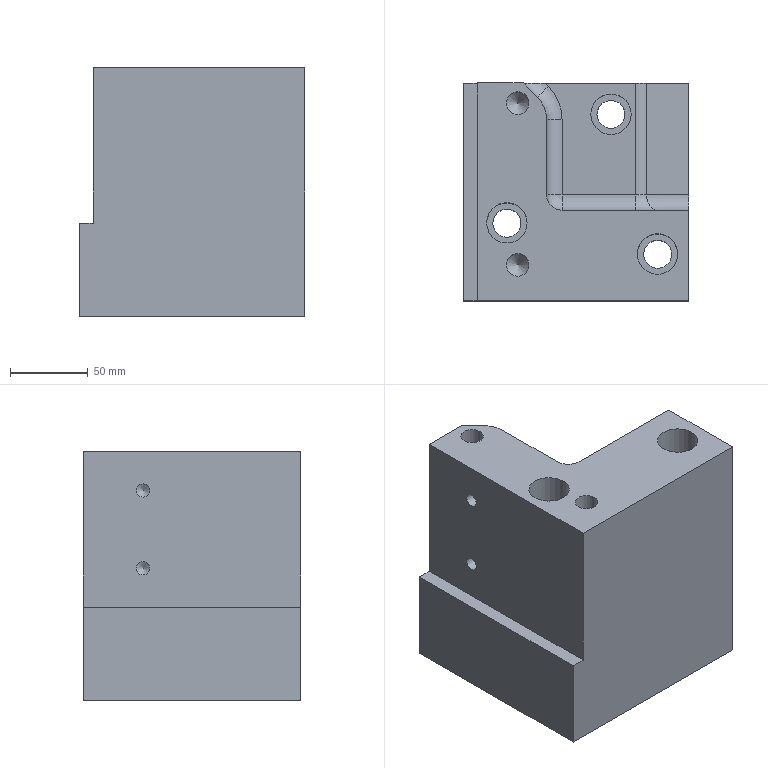Part | STEP file | lll_id86_x_t | 1 solid | 40 faces | box 145 x 140 x 160 mm | volume 2321770 mm3 | cylinder 17 | plane 16 | cone 4 | torus 2 | sphere 1 | commonest cylinder face diameters 20 x6 18.009 x3 26.008 x3 8.506 x2 14.506 x2 40 x1
STEP:
#1=CARTESIAN_POINT('',(2083.004,-384.047,65.));
#2=VERTEX_POINT('',#1);
#3=CARTESIAN_POINT('',(2070.,-384.047,65.));
#4=DIRECTION('',(0.,0.,-1.));
#5=DIRECTION('',(1.,0.,0.));
#6=AXIS2_PLACEMENT_3D('',#3,#4,#5);
#7=CIRCLE('',#6,13.004);
#8=EDGE_CURVE('',#2,#2,#7,.T.);
#9=ORIENTED_EDGE('',*,*,#8,.T.);
#10=EDGE_LOOP('',(#9));
#11=FACE_BOUND('',#10,.T.);
#12=CARTESIAN_POINT('',(1986.004,-364.047,65.));
#13=VERTEX_POINT('',#12);
#14=CARTESIAN_POINT('',(1973.,-364.047,65.));
#15=DIRECTION('',(0.,0.,-1.));
#16=DIRECTION('',(1.,0.,0.));
#17=AXIS2_PLACEMENT_3D('',#14,#15,#16);
#18=CIRCLE('',#17,13.004);
#19=EDGE_CURVE('',#13,#13,#18,.T.);
#20=ORIENTED_EDGE('',*,*,#19,.T.);
#21=EDGE_LOOP('',(#20));
#22=FACE_BOUND('',#21,.T.);
#23=CARTESIAN_POINT('',(1987.253,-287.047,65.));
#24=VERTEX_POINT('',#23);
#25=CARTESIAN_POINT('',(1980.,-287.047,65.));
#26=DIRECTION('',(0.,0.,1.));
#27=DIRECTION('',(1.,0.,0.));
#28=AXIS2_PLACEMENT_3D('',#25,#26,#27);
#29=CIRCLE('',#28,7.253);
#30=EDGE_CURVE('',#24,#24,#29,.T.);
#31=ORIENTED_EDGE('',*,*,#30,.F.);
#32=EDGE_LOOP('',(#31));
#33=FACE_BOUND('',#32,.T.);
#34=CARTESIAN_POINT('',(1987.253,-391.047,65.));
#35=VERTEX_POINT('',#34);
#36=CARTESIAN_POINT('',(1980.,-391.047,65.));
#37=DIRECTION('',(0.,0.,1.));
#38=DIRECTION('',(1.,0.,0.));
#39=AXIS2_PLACEMENT_3D('',#36,#37,#38);
#40=CIRCLE('',#39,7.253);
#41=EDGE_CURVE('',#35,#35,#40,.T.);
#42=ORIENTED_EDGE('',*,*,#41,.F.);
#43=EDGE_LOOP('',(#42));
#44=FACE_BOUND('',#43,.T.);
#45=CARTESIAN_POINT('',(1983.523,-274.047,65.));
#46=VERTEX_POINT('',#45);
#47=CARTESIAN_POINT('',(1992.666,-283.189,65.));
#48=VERTEX_POINT('',#47);
#49=CARTESIAN_POINT('',(1867.512,-158.035,65.));
#50=DIRECTION('',(0.7071,-0.7071,0.));
#51=VECTOR('',#50,1.);
#52=LINE('',#49,#51);
#53=EDGE_CURVE('',#46,#48,#52,.T.);
#54=ORIENTED_EDGE('',*,*,#53,.F.);
#55=CARTESIAN_POINT('',(1954.,-274.047,65.));
#56=VERTEX_POINT('',#55);
#57=CARTESIAN_POINT('',(1764.,-274.047,65.));
#58=DIRECTION('',(-1.,0.,0.));
#59=VECTOR('',#58,1.);
#60=LINE('',#57,#59);
#61=EDGE_CURVE('',#46,#56,#60,.T.);
#62=ORIENTED_EDGE('',*,*,#61,.T.);
#63=CARTESIAN_POINT('',(1954.,-414.047,65.));
#64=VERTEX_POINT('',#63);
#65=CARTESIAN_POINT('',(1954.,-261.547,65.));
#66=DIRECTION('',(0.,-1.,0.));
#67=VECTOR('',#66,1.);
#68=LINE('',#65,#67);
#69=EDGE_CURVE('',#56,#64,#68,.T.);
#70=ORIENTED_EDGE('',*,*,#69,.T.);
#71=CARTESIAN_POINT('',(2090.,-414.047,65.));
#72=VERTEX_POINT('',#71);
#73=CARTESIAN_POINT('',(1764.,-414.047,65.));
#74=DIRECTION('',(1.,0.,0.));
#75=VECTOR('',#74,1.);
#76=LINE('',#73,#75);
#77=EDGE_CURVE('',#64,#72,#76,.T.);
#78=ORIENTED_EDGE('',*,*,#77,.T.);
#79=CARTESIAN_POINT('',(2090.,-355.897,65.));
#80=VERTEX_POINT('',#79);
#81=CARTESIAN_POINT('',(2090.,-261.547,65.));
#82=DIRECTION('',(0.,1.,0.));
#83=VECTOR('',#82,1.);
#84=LINE('',#81,#83);
#85=EDGE_CURVE('',#72,#80,#84,.T.);
#86=ORIENTED_EDGE('',*,*,#85,.T.);
#87=CARTESIAN_POINT('',(2008.523,-355.897,65.));
#88=VERTEX_POINT('',#87);
#89=CARTESIAN_POINT('',(2073.192,-355.897,65.));
#90=DIRECTION('',(-1.,0.,0.));
#91=VECTOR('',#90,1.);
#92=LINE('',#89,#91);
#93=EDGE_CURVE('',#80,#88,#92,.T.);
#94=ORIENTED_EDGE('',*,*,#93,.T.);
#95=CARTESIAN_POINT('',(1998.523,-345.897,65.));
#96=VERTEX_POINT('',#95);
#97=CARTESIAN_POINT('',(2008.523,-345.897,65.));
#98=DIRECTION('',(0.,0.,1.));
#99=DIRECTION('',(1.,0.,0.));
#100=AXIS2_PLACEMENT_3D('',#97,#98,#99);
#101=CIRCLE('',#100,10.);
#102=EDGE_CURVE('',#96,#88,#101,.T.);
#103=ORIENTED_EDGE('',*,*,#102,.F.);
#104=CARTESIAN_POINT('',(1998.523,-297.331,65.));
#105=VERTEX_POINT('',#104);
#106=CARTESIAN_POINT('',(1998.523,-261.547,65.));
#107=DIRECTION('',(0.,1.,0.));
#108=VECTOR('',#107,1.);
#109=LINE('',#106,#108);
#110=EDGE_CURVE('',#96,#105,#109,.T.);
#111=ORIENTED_EDGE('',*,*,#110,.T.);
#112=CARTESIAN_POINT('',(1978.523,-297.331,65.));
#113=DIRECTION('',(0.,0.,-1.));
#114=DIRECTION('',(1.,0.,0.));
#115=AXIS2_PLACEMENT_3D('',#112,#113,#114);
#116=CIRCLE('',#115,20.);
#117=EDGE_CURVE('',#48,#105,#116,.T.);
#118=ORIENTED_EDGE('',*,*,#117,.F.);
#119=EDGE_LOOP('',(#54,#62,#70,#78,#86,#94,#103,#111,#118));
#120=FACE_BOUND('',#119,.T.);
#121=CARTESIAN_POINT('',(1764.,-261.547,65.));
#122=DIRECTION('',(0.,0.,1.));
#123=DIRECTION('',(-1.,0.,0.));
#124=AXIS2_PLACEMENT_3D('',#121,#122,#123);
#125=PLANE('',#124);
#126=ADVANCED_FACE('',(#11,#22,#33,#44,#120),#125,.T.);
#127=CARTESIAN_POINT('',(1945.,-274.047,-95.));
#128=VERTEX_POINT('',#127);
#129=CARTESIAN_POINT('',(1945.,-414.047,-95.));
#130=VERTEX_POINT('',#129);
#131=CARTESIAN_POINT('',(1945.,5.,-95.));
#132=DIRECTION('',(0.,-1.,0.));
#133=VECTOR('',#132,1.);
#134=LINE('',#131,#133);
#135=EDGE_CURVE('',#128,#130,#134,.T.);
#136=ORIENTED_EDGE('',*,*,#135,.T.);
#137=CARTESIAN_POINT('',(1945.,-414.047,-35.));
#138=VERTEX_POINT('',#137);
#139=CARTESIAN_POINT('',(1945.,-414.047,-690.));
#140=DIRECTION('',(0.,0.,-1.));
#141=VECTOR('',#140,1.);
#142=LINE('',#139,#141);
#143=EDGE_CURVE('',#138,#130,#142,.T.);
#144=ORIENTED_EDGE('',*,*,#143,.F.);
#145=CARTESIAN_POINT('',(1945.,-274.047,-35.));
#146=VERTEX_POINT('',#145);
#147=CARTESIAN_POINT('',(1945.,6.,-35.));
#148=DIRECTION('',(0.,-1.,0.));
#149=VECTOR('',#148,1.);
#150=LINE('',#147,#149);
#151=EDGE_CURVE('',#146,#138,#150,.T.);
#152=ORIENTED_EDGE('',*,*,#151,.F.);
#153=CARTESIAN_POINT('',(1945.,-274.047,-690.));
#154=DIRECTION('',(0.,0.,1.));
#155=VECTOR('',#154,1.);
#156=LINE('',#153,#155);
#157=EDGE_CURVE('',#128,#146,#156,.T.);
#158=ORIENTED_EDGE('',*,*,#157,.F.);
#159=EDGE_LOOP('',(#136,#144,#152,#158));
#160=FACE_OUTER_BOUND('',#159,.T.);
#161=CARTESIAN_POINT('',(1945.,5.,-690.));
#162=DIRECTION('',(1.,0.,0.));
#163=DIRECTION('',(0.,0.,1.));
#164=AXIS2_PLACEMENT_3D('',#161,#162,#163);
#165=PLANE('',#164);
#166=ADVANCED_FACE('',(#160),#165,.F.);
#167=CARTESIAN_POINT('',(2090.,-355.897,-25.858));
#168=VERTEX_POINT('',#167);
#169=CARTESIAN_POINT('',(2090.,-355.897,-120.));
#170=DIRECTION('',(0.,0.,-1.));
#171=VECTOR('',#170,1.);
#172=LINE('',#169,#171);
#173=EDGE_CURVE('',#80,#168,#172,.T.);
#174=ORIENTED_EDGE('',*,*,#173,.F.);
#175=ORIENTED_EDGE('',*,*,#85,.F.);
#176=CARTESIAN_POINT('',(2090.,-414.047,-95.));
#177=VERTEX_POINT('',#176);
#178=CARTESIAN_POINT('',(2090.,-414.047,-120.));
#179=DIRECTION('',(0.,0.,1.));
#180=VECTOR('',#179,1.);
#181=LINE('',#178,#180);
#182=EDGE_CURVE('',#177,#72,#181,.T.);
#183=ORIENTED_EDGE('',*,*,#182,.F.);
#184=CARTESIAN_POINT('',(2090.,-274.047,-95.));
#185=VERTEX_POINT('',#184);
#186=CARTESIAN_POINT('',(2090.,-261.547,-95.));
#187=DIRECTION('',(0.,-1.,0.));
#188=VECTOR('',#187,1.);
#189=LINE('',#186,#188);
#190=EDGE_CURVE('',#185,#177,#189,.T.);
#191=ORIENTED_EDGE('',*,*,#190,.F.);
#192=CARTESIAN_POINT('',(2090.,-274.047,-40.));
#193=VERTEX_POINT('',#192);
#194=CARTESIAN_POINT('',(2090.,-274.047,-120.));
#195=DIRECTION('',(0.,0.,-1.));
#196=VECTOR('',#195,1.);
#197=LINE('',#194,#196);
#198=EDGE_CURVE('',#193,#185,#197,.T.);
#199=ORIENTED_EDGE('',*,*,#198,.F.);
#200=CARTESIAN_POINT('',(2090.,-345.897,-40.));
#201=VERTEX_POINT('',#200);
#202=CARTESIAN_POINT('',(2090.,-274.047,-40.));
#203=DIRECTION('',(0.,1.,0.));
#204=VECTOR('',#203,1.);
#205=LINE('',#202,#204);
#206=EDGE_CURVE('',#201,#193,#205,.T.);
#207=ORIENTED_EDGE('',*,*,#206,.F.);
#208=CARTESIAN_POINT('',(2090.,-345.897,-25.858));
#209=DIRECTION('',(1.,0.,0.));
#210=DIRECTION('',(0.,0.,-1.));
#211=AXIS2_PLACEMENT_3D('',#208,#209,#210);
#212=ELLIPSE('',#211,14.142,10.);
#213=EDGE_CURVE('',#168,#201,#212,.T.);
#214=ORIENTED_EDGE('',*,*,#213,.F.);
#215=EDGE_LOOP('',(#174,#175,#183,#191,#199,#207,#214));
#216=FACE_OUTER_BOUND('',#215,.T.);
#217=CARTESIAN_POINT('',(2090.,-261.547,-120.));
#218=DIRECTION('',(1.,0.,0.));
#219=DIRECTION('',(0.,0.,1.));
#220=AXIS2_PLACEMENT_3D('',#217,#218,#219);
#221=PLANE('',#220);
#222=ADVANCED_FACE('',(#216),#221,.T.);
#223=CARTESIAN_POINT('',(2062.929,-274.047,-12.929));
#224=VERTEX_POINT('',#223);
#225=CARTESIAN_POINT('',(2090.,-274.047,-40.));
#226=DIRECTION('',(-0.7071,0.,0.7071));
#227=VECTOR('',#226,1.);
#228=LINE('',#225,#227);
#229=EDGE_CURVE('',#193,#224,#228,.T.);
#230=ORIENTED_EDGE('',*,*,#229,.F.);
#231=ORIENTED_EDGE('',*,*,#198,.T.);
#232=CARTESIAN_POINT('',(1764.,-274.047,-95.));
#233=DIRECTION('',(-1.,0.,0.));
#234=VECTOR('',#233,1.);
#235=LINE('',#232,#234);
#236=EDGE_CURVE('',#185,#128,#235,.T.);
#237=ORIENTED_EDGE('',*,*,#236,.T.);
#238=ORIENTED_EDGE('',*,*,#157,.T.);
#239=CARTESIAN_POINT('',(1954.,-274.047,-35.));
#240=VERTEX_POINT('',#239);
#241=CARTESIAN_POINT('',(1241.435,-274.047,-35.));
#242=DIRECTION('',(1.,0.,0.));
#243=VECTOR('',#242,1.);
#244=LINE('',#241,#243);
#245=EDGE_CURVE('',#146,#240,#244,.T.);
#246=ORIENTED_EDGE('',*,*,#245,.T.);
#247=CARTESIAN_POINT('',(1954.,-274.047,131.231));
#248=DIRECTION('',(0.,0.,1.));
#249=VECTOR('',#248,1.);
#250=LINE('',#247,#249);
#251=EDGE_CURVE('',#240,#56,#250,.T.);
#252=ORIENTED_EDGE('',*,*,#251,.T.);
#253=ORIENTED_EDGE('',*,*,#61,.F.);
#254=CARTESIAN_POINT('',(1983.523,-274.047,0.));
#255=VERTEX_POINT('',#254);
#256=CARTESIAN_POINT('',(1983.523,-274.047,-3.));
#257=DIRECTION('',(0.,0.,1.));
#258=VECTOR('',#257,1.);
#259=LINE('',#256,#258);
#260=EDGE_CURVE('',#255,#46,#259,.T.);
#261=ORIENTED_EDGE('',*,*,#260,.F.);
#262=CARTESIAN_POINT('',(1997.666,-274.047,-10.));
#263=VERTEX_POINT('',#262);
#264=CARTESIAN_POINT('',(1997.666,-274.047,0.));
#265=DIRECTION('',(0.,1.,0.));
#266=DIRECTION('',(1.,0.,0.));
#267=AXIS2_PLACEMENT_3D('',#264,#265,#266);
#268=ELLIPSE('',#267,14.142,10.);
#269=EDGE_CURVE('',#263,#255,#268,.T.);
#270=ORIENTED_EDGE('',*,*,#269,.F.);
#271=CARTESIAN_POINT('',(2055.858,-274.047,-10.));
#272=VERTEX_POINT('',#271);
#273=CARTESIAN_POINT('',(1814.,-274.047,-10.));
#274=DIRECTION('',(1.,0.,0.));
#275=VECTOR('',#274,1.);
#276=LINE('',#273,#275);
#277=EDGE_CURVE('',#263,#272,#276,.T.);
#278=ORIENTED_EDGE('',*,*,#277,.T.);
#279=CARTESIAN_POINT('',(2055.858,-274.047,-20.));
#280=DIRECTION('',(0.,-1.,0.));
#281=DIRECTION('',(0.,0.,1.));
#282=AXIS2_PLACEMENT_3D('',#279,#280,#281);
#283=CIRCLE('',#282,10.);
#284=EDGE_CURVE('',#224,#272,#283,.T.);
#285=ORIENTED_EDGE('',*,*,#284,.F.);
#286=EDGE_LOOP('',(#230,#231,#237,#238,#246,#252,#253,#261,#270,#278,#285));
#287=FACE_OUTER_BOUND('',#286,.T.);
#288=CARTESIAN_POINT('',(1764.,-274.047,-105.));
#289=DIRECTION('',(0.,-1.,0.));
#290=DIRECTION('',(0.,0.,-1.));
#291=AXIS2_PLACEMENT_3D('',#288,#289,#290);
#292=PLANE('',#291);
#293=ADVANCED_FACE('',(#287),#292,.F.);
#294=CARTESIAN_POINT('',(1954.,-312.547,-14.253));
#295=VERTEX_POINT('',#294);
#296=CARTESIAN_POINT('',(1954.,-312.547,-10.));
#297=DIRECTION('',(1.,0.,0.));
#298=DIRECTION('',(0.,0.,-1.));
#299=AXIS2_PLACEMENT_3D('',#296,#297,#298);
#300=CIRCLE('',#299,4.253);
#301=EDGE_CURVE('',#295,#295,#300,.T.);
#302=ORIENTED_EDGE('',*,*,#301,.T.);
#303=EDGE_LOOP('',(#302));
#304=FACE_BOUND('',#303,.T.);
#305=CARTESIAN_POINT('',(1954.,-312.547,35.747));
#306=VERTEX_POINT('',#305);
#307=CARTESIAN_POINT('',(1954.,-312.547,40.));
#308=DIRECTION('',(1.,0.,0.));
#309=DIRECTION('',(0.,0.,-1.));
#310=AXIS2_PLACEMENT_3D('',#307,#308,#309);
#311=CIRCLE('',#310,4.253);
#312=EDGE_CURVE('',#306,#306,#311,.T.);
#313=ORIENTED_EDGE('',*,*,#312,.T.);
#314=EDGE_LOOP('',(#313));
#315=FACE_BOUND('',#314,.T.);
#316=CARTESIAN_POINT('',(1954.,-414.047,-35.));
#317=VERTEX_POINT('',#316);
#318=CARTESIAN_POINT('',(1954.,-267.323,-35.));
#319=DIRECTION('',(0.,-1.,0.));
#320=VECTOR('',#319,1.);
#321=LINE('',#318,#320);
#322=EDGE_CURVE('',#240,#317,#321,.T.);
#323=ORIENTED_EDGE('',*,*,#322,.T.);
#324=CARTESIAN_POINT('',(1954.,-414.047,-120.));
#325=DIRECTION('',(0.,0.,-1.));
#326=VECTOR('',#325,1.);
#327=LINE('',#324,#326);
#328=EDGE_CURVE('',#64,#317,#327,.T.);
#329=ORIENTED_EDGE('',*,*,#328,.F.);
#330=ORIENTED_EDGE('',*,*,#69,.F.);
#331=ORIENTED_EDGE('',*,*,#251,.F.);
#332=EDGE_LOOP('',(#323,#329,#330,#331));
#333=FACE_BOUND('',#332,.T.);
#334=CARTESIAN_POINT('',(1954.,-267.323,131.231));
#335=DIRECTION('',(1.,0.,0.));
#336=DIRECTION('',(0.,0.,1.));
#337=AXIS2_PLACEMENT_3D('',#334,#335,#336);
#338=PLANE('',#337);
#339=ADVANCED_FACE('',(#304,#315,#333),#338,.F.);
#340=ORIENTED_EDGE('',*,*,#151,.T.);
#341=CARTESIAN_POINT('',(1241.435,-414.047,-35.));
#342=DIRECTION('',(1.,0.,0.));
#343=VECTOR('',#342,1.);
#344=LINE('',#341,#343);
#345=EDGE_CURVE('',#138,#317,#344,.T.);
#346=ORIENTED_EDGE('',*,*,#345,.T.);
#347=ORIENTED_EDGE('',*,*,#322,.F.);
#348=ORIENTED_EDGE('',*,*,#245,.F.);
#349=EDGE_LOOP('',(#340,#346,#347,#348));
#350=FACE_OUTER_BOUND('',#349,.T.);
#351=CARTESIAN_POINT('',(1241.435,6.,-35.));
#352=DIRECTION('',(0.,0.,1.));
#353=DIRECTION('',(1.,0.,0.));
#354=AXIS2_PLACEMENT_3D('',#351,#352,#353);
#355=PLANE('',#354);
#356=ADVANCED_FACE('',(#350),#355,.T.);
#357=ORIENTED_EDGE('',*,*,#328,.T.);
#358=ORIENTED_EDGE('',*,*,#345,.F.);
#359=ORIENTED_EDGE('',*,*,#143,.T.);
#360=CARTESIAN_POINT('',(2092.435,-414.047,-95.));
#361=DIRECTION('',(-1.,0.,0.));
#362=VECTOR('',#361,1.);
#363=LINE('',#360,#362);
#364=EDGE_CURVE('',#177,#130,#363,.T.);
#365=ORIENTED_EDGE('',*,*,#364,.F.);
#366=ORIENTED_EDGE('',*,*,#182,.T.);
#367=ORIENTED_EDGE('',*,*,#77,.F.);
#368=EDGE_LOOP('',(#357,#358,#359,#365,#366,#367));
#369=FACE_OUTER_BOUND('',#368,.T.);
#370=CARTESIAN_POINT('',(1764.,-414.047,-120.));
#371=DIRECTION('',(0.,-1.,0.));
#372=DIRECTION('',(0.,0.,-1.));
#373=AXIS2_PLACEMENT_3D('',#370,#371,#372);
#374=PLANE('',#373);
#375=ADVANCED_FACE('',(#369),#374,.T.);
#376=CARTESIAN_POINT('',(2049.005,-294.047,-95.));
#377=VERTEX_POINT('',#376);
#378=CARTESIAN_POINT('',(2040.,-294.047,-95.));
#379=DIRECTION('',(0.,0.,1.));
#380=DIRECTION('',(1.,0.,0.));
#381=AXIS2_PLACEMENT_3D('',#378,#379,#380);
#382=CIRCLE('',#381,9.005);
#383=EDGE_CURVE('',#377,#377,#382,.T.);
#384=ORIENTED_EDGE('',*,*,#383,.T.);
#385=EDGE_LOOP('',(#384));
#386=FACE_BOUND('',#385,.T.);
#387=CARTESIAN_POINT('',(1982.005,-364.047,-95.));
#388=VERTEX_POINT('',#387);
#389=CARTESIAN_POINT('',(1973.,-364.047,-95.));
#390=DIRECTION('',(0.,0.,1.));
#391=DIRECTION('',(1.,0.,0.));
#392=AXIS2_PLACEMENT_3D('',#389,#390,#391);
#393=CIRCLE('',#392,9.005);
#394=EDGE_CURVE('',#388,#388,#393,.T.);
#395=ORIENTED_EDGE('',*,*,#394,.T.);
#396=EDGE_LOOP('',(#395));
#397=FACE_BOUND('',#396,.T.);
#398=CARTESIAN_POINT('',(2079.005,-384.047,-95.));
#399=VERTEX_POINT('',#398);
#400=CARTESIAN_POINT('',(2070.,-384.047,-95.));
#401=DIRECTION('',(0.,0.,1.));
#402=DIRECTION('',(1.,0.,0.));
#403=AXIS2_PLACEMENT_3D('',#400,#401,#402);
#404=CIRCLE('',#403,9.005);
#405=EDGE_CURVE('',#399,#399,#404,.T.);
#406=ORIENTED_EDGE('',*,*,#405,.T.);
#407=EDGE_LOOP('',(#406));
#408=FACE_BOUND('',#407,.T.);
#409=ORIENTED_EDGE('',*,*,#236,.F.);
#410=ORIENTED_EDGE('',*,*,#190,.T.);
#411=ORIENTED_EDGE('',*,*,#364,.T.);
#412=ORIENTED_EDGE('',*,*,#135,.F.);
#413=EDGE_LOOP('',(#409,#410,#411,#412));
#414=FACE_BOUND('',#413,.T.);
#415=CARTESIAN_POINT('',(2092.435,10.,-95.));
#416=DIRECTION('',(0.,0.,1.));
#417=DIRECTION('',(1.,0.,0.));
#418=AXIS2_PLACEMENT_3D('',#415,#416,#417);
#419=PLANE('',#418);
#420=ADVANCED_FACE('',(#386,#397,#408,#414),#419,.F.);
#421=CARTESIAN_POINT('',(1984.,-312.547,35.747));
#422=VERTEX_POINT('',#421);
#423=CARTESIAN_POINT('',(1984.,-312.547,40.));
#424=DIRECTION('',(-1.,0.,0.));
#425=DIRECTION('',(0.,0.,-1.));
#426=AXIS2_PLACEMENT_3D('',#423,#424,#425);
#427=CIRCLE('',#426,4.253);
#428=EDGE_CURVE('',#422,#422,#427,.T.);
#429=ORIENTED_EDGE('',*,*,#428,.T.);
#430=EDGE_LOOP('',(#429));
#431=FACE_BOUND('',#430,.T.);
#432=CARTESIAN_POINT('',(1986.555,-312.547,40.));
#433=VERTEX_POINT('',#432);
#434=VERTEX_LOOP('',#433);
#435=FACE_BOUND('',#434,.T.);
#436=CARTESIAN_POINT('',(1984.,-312.547,40.));
#437=DIRECTION('',(-1.,0.,0.));
#438=DIRECTION('',(0.,0.,1.));
#439=AXIS2_PLACEMENT_3D('',#436,#437,#438);
#440=CONICAL_SURFACE('',#439,4.253,59.);
#441=ADVANCED_FACE('',(#431,#435),#440,.F.);
#442=ORIENTED_EDGE('',*,*,#428,.F.);
#443=EDGE_LOOP('',(#442));
#444=FACE_BOUND('',#443,.T.);
#445=ORIENTED_EDGE('',*,*,#312,.F.);
#446=EDGE_LOOP('',(#445));
#447=FACE_BOUND('',#446,.T.);
#448=CARTESIAN_POINT('',(1954.,-312.547,40.));
#449=DIRECTION('',(1.,0.,0.));
#450=DIRECTION('',(0.,0.,-1.));
#451=AXIS2_PLACEMENT_3D('',#448,#449,#450);
#452=CYLINDRICAL_SURFACE('',#451,4.253);
#453=ADVANCED_FACE('',(#444,#447),#452,.F.);
#454=CARTESIAN_POINT('',(1984.,-312.547,-14.253));
#455=VERTEX_POINT('',#454);
#456=CARTESIAN_POINT('',(1984.,-312.547,-10.));
#457=DIRECTION('',(-1.,0.,0.));
#458=DIRECTION('',(0.,0.,-1.));
#459=AXIS2_PLACEMENT_3D('',#456,#457,#458);
#460=CIRCLE('',#459,4.253);
#461=EDGE_CURVE('',#455,#455,#460,.T.);
#462=ORIENTED_EDGE('',*,*,#461,.T.);
#463=EDGE_LOOP('',(#462));
#464=FACE_BOUND('',#463,.T.);
#465=CARTESIAN_POINT('',(1986.555,-312.547,-10.));
#466=VERTEX_POINT('',#465);
#467=VERTEX_LOOP('',#466);
#468=FACE_BOUND('',#467,.T.);
#469=CARTESIAN_POINT('',(1984.,-312.547,-10.));
#470=DIRECTION('',(-1.,0.,0.));
#471=DIRECTION('',(0.,0.,1.));
#472=AXIS2_PLACEMENT_3D('',#469,#470,#471);
#473=CONICAL_SURFACE('',#472,4.253,59.);
#474=ADVANCED_FACE('',(#464,#468),#473,.F.);
#475=ORIENTED_EDGE('',*,*,#461,.F.);
#476=EDGE_LOOP('',(#475));
#477=FACE_BOUND('',#476,.T.);
#478=ORIENTED_EDGE('',*,*,#301,.F.);
#479=EDGE_LOOP('',(#478));
#480=FACE_BOUND('',#479,.T.);
#481=CARTESIAN_POINT('',(1954.,-312.547,-10.));
#482=DIRECTION('',(1.,0.,0.));
#483=DIRECTION('',(0.,0.,-1.));
#484=AXIS2_PLACEMENT_3D('',#481,#482,#483);
#485=CYLINDRICAL_SURFACE('',#484,4.253);
#486=ADVANCED_FACE('',(#477,#480),#485,.F.);
#487=CARTESIAN_POINT('',(2060.995,-384.047,-55.));
#488=VERTEX_POINT('',#487);
#489=CARTESIAN_POINT('',(2070.,-384.047,-55.));
#490=DIRECTION('',(0.,0.,-1.));
#491=DIRECTION('',(-1.,0.,0.));
#492=AXIS2_PLACEMENT_3D('',#489,#490,#491);
#493=CIRCLE('',#492,9.005);
#494=EDGE_CURVE('',#488,#488,#493,.T.);
#495=ORIENTED_EDGE('',*,*,#494,.F.);
#496=EDGE_LOOP('',(#495));
#497=FACE_BOUND('',#496,.T.);
#498=ORIENTED_EDGE('',*,*,#405,.F.);
#499=EDGE_LOOP('',(#498));
#500=FACE_BOUND('',#499,.T.);
#501=CARTESIAN_POINT('',(2070.,-384.047,67.));
#502=DIRECTION('',(0.,0.,-1.));
#503=DIRECTION('',(1.,0.,0.));
#504=AXIS2_PLACEMENT_3D('',#501,#502,#503);
#505=CYLINDRICAL_SURFACE('',#504,9.005);
#506=ADVANCED_FACE('',(#497,#500),#505,.F.);
#507=ORIENTED_EDGE('',*,*,#494,.T.);
#508=EDGE_LOOP('',(#507));
#509=FACE_BOUND('',#508,.T.);
#510=CARTESIAN_POINT('',(2083.004,-384.047,-55.));
#511=VERTEX_POINT('',#510);
#512=CARTESIAN_POINT('',(2070.,-384.047,-55.));
#513=DIRECTION('',(0.,0.,-1.));
#514=DIRECTION('',(1.,0.,0.));
#515=AXIS2_PLACEMENT_3D('',#512,#513,#514);
#516=CIRCLE('',#515,13.004);
#517=EDGE_CURVE('',#511,#511,#516,.T.);
#518=ORIENTED_EDGE('',*,*,#517,.F.);
#519=EDGE_LOOP('',(#518));
#520=FACE_BOUND('',#519,.T.);
#521=CARTESIAN_POINT('',(2070.,-384.047,-55.));
#522=DIRECTION('',(0.,0.,-1.));
#523=DIRECTION('',(-1.,0.,0.));
#524=AXIS2_PLACEMENT_3D('',#521,#522,#523);
#525=PLANE('',#524);
#526=ADVANCED_FACE('',(#509,#520),#525,.F.);
#527=ORIENTED_EDGE('',*,*,#517,.T.);
#528=EDGE_LOOP('',(#527));
#529=FACE_BOUND('',#528,.T.);
#530=ORIENTED_EDGE('',*,*,#8,.F.);
#531=EDGE_LOOP('',(#530));
#532=FACE_BOUND('',#531,.T.);
#533=CARTESIAN_POINT('',(2070.,-384.047,65.));
#534=DIRECTION('',(0.,0.,-1.));
#535=DIRECTION('',(1.,0.,0.));
#536=AXIS2_PLACEMENT_3D('',#533,#534,#535);
#537=CYLINDRICAL_SURFACE('',#536,13.004);
#538=ADVANCED_FACE('',(#529,#532),#537,.F.);
#539=CARTESIAN_POINT('',(1963.995,-364.047,-55.));
#540=VERTEX_POINT('',#539);
#541=CARTESIAN_POINT('',(1973.,-364.047,-55.));
#542=DIRECTION('',(0.,0.,-1.));
#543=DIRECTION('',(-1.,0.,0.));
#544=AXIS2_PLACEMENT_3D('',#541,#542,#543);
#545=CIRCLE('',#544,9.005);
#546=EDGE_CURVE('',#540,#540,#545,.T.);
#547=ORIENTED_EDGE('',*,*,#546,.F.);
#548=EDGE_LOOP('',(#547));
#549=FACE_BOUND('',#548,.T.);
#550=ORIENTED_EDGE('',*,*,#394,.F.);
#551=EDGE_LOOP('',(#550));
#552=FACE_BOUND('',#551,.T.);
#553=CARTESIAN_POINT('',(1973.,-364.047,67.));
#554=DIRECTION('',(0.,0.,-1.));
#555=DIRECTION('',(1.,0.,0.));
#556=AXIS2_PLACEMENT_3D('',#553,#554,#555);
#557=CYLINDRICAL_SURFACE('',#556,9.005);
#558=ADVANCED_FACE('',(#549,#552),#557,.F.);
#559=ORIENTED_EDGE('',*,*,#546,.T.);
#560=EDGE_LOOP('',(#559));
#561=FACE_BOUND('',#560,.T.);
#562=CARTESIAN_POINT('',(1986.004,-364.047,-55.));
#563=VERTEX_POINT('',#562);
#564=CARTESIAN_POINT('',(1973.,-364.047,-55.));
#565=DIRECTION('',(0.,0.,-1.));
#566=DIRECTION('',(1.,0.,0.));
#567=AXIS2_PLACEMENT_3D('',#564,#565,#566);
#568=CIRCLE('',#567,13.004);
#569=EDGE_CURVE('',#563,#563,#568,.T.);
#570=ORIENTED_EDGE('',*,*,#569,.F.);
#571=EDGE_LOOP('',(#570));
#572=FACE_BOUND('',#571,.T.);
#573=CARTESIAN_POINT('',(1973.,-364.047,-55.));
#574=DIRECTION('',(0.,0.,-1.));
#575=DIRECTION('',(-1.,0.,0.));
#576=AXIS2_PLACEMENT_3D('',#573,#574,#575);
#577=PLANE('',#576);
#578=ADVANCED_FACE('',(#561,#572),#577,.F.);
#579=ORIENTED_EDGE('',*,*,#569,.T.);
#580=EDGE_LOOP('',(#579));
#581=FACE_BOUND('',#580,.T.);
#582=ORIENTED_EDGE('',*,*,#19,.F.);
#583=EDGE_LOOP('',(#582));
#584=FACE_BOUND('',#583,.T.);
#585=CARTESIAN_POINT('',(1973.,-364.047,65.));
#586=DIRECTION('',(0.,0.,-1.));
#587=DIRECTION('',(1.,0.,0.));
#588=AXIS2_PLACEMENT_3D('',#585,#586,#587);
#589=CYLINDRICAL_SURFACE('',#588,13.004);
#590=ADVANCED_FACE('',(#581,#584),#589,.F.);
#591=CARTESIAN_POINT('',(2030.995,-294.047,-55.));
#592=VERTEX_POINT('',#591);
#593=CARTESIAN_POINT('',(2040.,-294.047,-55.));
#594=DIRECTION('',(0.,0.,-1.));
#595=DIRECTION('',(-1.,0.,0.));
#596=AXIS2_PLACEMENT_3D('',#593,#594,#595);
#597=CIRCLE('',#596,9.005);
#598=EDGE_CURVE('',#592,#592,#597,.T.);
#599=ORIENTED_EDGE('',*,*,#598,.F.);
#600=EDGE_LOOP('',(#599));
#601=FACE_BOUND('',#600,.T.);
#602=ORIENTED_EDGE('',*,*,#383,.F.);
#603=EDGE_LOOP('',(#602));
#604=FACE_BOUND('',#603,.T.);
#605=CARTESIAN_POINT('',(2040.,-294.047,67.));
#606=DIRECTION('',(0.,0.,-1.));
#607=DIRECTION('',(1.,0.,0.));
#608=AXIS2_PLACEMENT_3D('',#605,#606,#607);
#609=CYLINDRICAL_SURFACE('',#608,9.005);
#610=ADVANCED_FACE('',(#601,#604),#609,.F.);
#611=ORIENTED_EDGE('',*,*,#598,.T.);
#612=EDGE_LOOP('',(#611));
#613=FACE_BOUND('',#612,.T.);
#614=CARTESIAN_POINT('',(2053.004,-294.047,-55.));
#615=VERTEX_POINT('',#614);
#616=CARTESIAN_POINT('',(2040.,-294.047,-55.));
#617=DIRECTION('',(0.,0.,-1.));
#618=DIRECTION('',(1.,0.,0.));
#619=AXIS2_PLACEMENT_3D('',#616,#617,#618);
#620=CIRCLE('',#619,13.004);
#621=EDGE_CURVE('',#615,#615,#620,.T.);
#622=ORIENTED_EDGE('',*,*,#621,.F.);
#623=EDGE_LOOP('',(#622));
#624=FACE_BOUND('',#623,.T.);
#625=CARTESIAN_POINT('',(2040.,-294.047,-55.));
#626=DIRECTION('',(0.,0.,-1.));
#627=DIRECTION('',(-1.,0.,0.));
#628=AXIS2_PLACEMENT_3D('',#625,#626,#627);
#629=PLANE('',#628);
#630=ADVANCED_FACE('',(#613,#624),#629,.F.);
#631=CARTESIAN_POINT('',(2026.996,-294.047,-10.));
#632=VERTEX_POINT('',#631);
#633=CARTESIAN_POINT('',(2040.,-294.047,-10.));
#634=DIRECTION('',(0.,0.,1.));
#635=DIRECTION('',(-1.,0.,0.));
#636=AXIS2_PLACEMENT_3D('',#633,#634,#635);
#637=CIRCLE('',#636,13.004);
#638=EDGE_CURVE('',#632,#632,#637,.T.);
#639=ORIENTED_EDGE('',*,*,#638,.T.);
#640=EDGE_LOOP('',(#639));
#641=FACE_BOUND('',#640,.T.);
#642=ORIENTED_EDGE('',*,*,#621,.T.);
#643=EDGE_LOOP('',(#642));
#644=FACE_BOUND('',#643,.T.);
#645=CARTESIAN_POINT('',(2040.,-294.047,65.));
#646=DIRECTION('',(0.,0.,-1.));
#647=DIRECTION('',(1.,0.,0.));
#648=AXIS2_PLACEMENT_3D('',#645,#646,#647);
#649=CYLINDRICAL_SURFACE('',#648,13.004);
#650=ADVANCED_FACE('',(#641,#644),#649,.F.);
#651=ORIENTED_EDGE('',*,*,#30,.T.);
#652=EDGE_LOOP('',(#651));
#653=FACE_BOUND('',#652,.T.);
#654=CARTESIAN_POINT('',(1972.747,-287.047,29.247));
#655=VERTEX_POINT('',#654);
#656=CARTESIAN_POINT('',(1980.,-287.047,29.247));
#657=DIRECTION('',(0.,0.,-1.));
#658=DIRECTION('',(-1.,0.,0.));
#659=AXIS2_PLACEMENT_3D('',#656,#657,#658);
#660=CIRCLE('',#659,7.253);
#661=EDGE_CURVE('',#655,#655,#660,.T.);
#662=ORIENTED_EDGE('',*,*,#661,.T.);
#663=EDGE_LOOP('',(#662));
#664=FACE_BOUND('',#663,.T.);
#665=CARTESIAN_POINT('',(1980.,-287.047,67.));
#666=DIRECTION('',(0.,0.,-1.));
#667=DIRECTION('',(1.,0.,0.));
#668=AXIS2_PLACEMENT_3D('',#665,#666,#667);
#669=CYLINDRICAL_SURFACE('',#668,7.253);
#670=ADVANCED_FACE('',(#653,#664),#669,.F.);
#671=CARTESIAN_POINT('',(1980.,-287.047,21.994));
#672=VERTEX_POINT('',#671);
#673=VERTEX_LOOP('',#672);
#674=FACE_BOUND('',#673,.T.);
#675=ORIENTED_EDGE('',*,*,#661,.F.);
#676=EDGE_LOOP('',(#675));
#677=FACE_BOUND('',#676,.T.);
#678=CARTESIAN_POINT('',(1980.,-287.047,29.247));
#679=DIRECTION('',(0.,0.,1.));
#680=DIRECTION('',(1.,0.,0.));
#681=AXIS2_PLACEMENT_3D('',#678,#679,#680);
#682=CONICAL_SURFACE('',#681,7.253,45.);
#683=ADVANCED_FACE('',(#674,#677),#682,.F.);
#684=ORIENTED_EDGE('',*,*,#41,.T.);
#685=EDGE_LOOP('',(#684));
#686=FACE_BOUND('',#685,.T.);
#687=CARTESIAN_POINT('',(1972.747,-391.047,29.247));
#688=VERTEX_POINT('',#687);
#689=CARTESIAN_POINT('',(1980.,-391.047,29.247));
#690=DIRECTION('',(0.,0.,1.));
#691=DIRECTION('',(-1.,0.,0.));
#692=AXIS2_PLACEMENT_3D('',#689,#690,#691);
#693=CIRCLE('',#692,7.253);
#694=EDGE_CURVE('',#688,#688,#693,.T.);
#695=ORIENTED_EDGE('',*,*,#694,.F.);
#696=EDGE_LOOP('',(#695));
#697=FACE_BOUND('',#696,.T.);
#698=CARTESIAN_POINT('',(1980.,-391.047,67.));
#699=DIRECTION('',(0.,0.,-1.));
#700=DIRECTION('',(1.,0.,0.));
#701=AXIS2_PLACEMENT_3D('',#698,#699,#700);
#702=CYLINDRICAL_SURFACE('',#701,7.253);
#703=ADVANCED_FACE('',(#686,#697),#702,.F.);
#704=CARTESIAN_POINT('',(1980.,-391.047,21.994));
#705=VERTEX_POINT('',#704);
#706=VERTEX_LOOP('',#705);
#707=FACE_BOUND('',#706,.T.);
#708=ORIENTED_EDGE('',*,*,#694,.T.);
#709=EDGE_LOOP('',(#708));
#710=FACE_BOUND('',#709,.T.);
#711=CARTESIAN_POINT('',(1980.,-391.047,29.247));
#712=DIRECTION('',(0.,0.,1.));
#713=DIRECTION('',(1.,0.,0.));
#714=AXIS2_PLACEMENT_3D('',#711,#712,#713);
#715=CONICAL_SURFACE('',#714,7.253,45.);
#716=ADVANCED_FACE('',(#707,#710),#715,.F.);
#717=CARTESIAN_POINT('',(1998.523,-297.331,0.));
#718=VERTEX_POINT('',#717);
#719=CARTESIAN_POINT('',(1998.523,-297.331,-3.));
#720=DIRECTION('',(0.,0.,-1.));
#721=VECTOR('',#720,1.);
#722=LINE('',#719,#721);
#723=EDGE_CURVE('',#105,#718,#722,.T.);
#724=ORIENTED_EDGE('',*,*,#723,.F.);
#725=ORIENTED_EDGE('',*,*,#110,.F.);
#726=CARTESIAN_POINT('',(1998.523,-345.897,0.));
#727=VERTEX_POINT('',#726);
#728=CARTESIAN_POINT('',(1998.523,-345.897,65.));
#729=DIRECTION('',(0.,0.,1.));
#730=VECTOR('',#729,1.);
#731=LINE('',#728,#730);
#732=EDGE_CURVE('',#727,#96,#731,.T.);
#733=ORIENTED_EDGE('',*,*,#732,.F.);
#734=CARTESIAN_POINT('',(1998.523,-345.897,0.));
#735=DIRECTION('',(0.,-1.,0.));
#736=VECTOR('',#735,1.);
#737=LINE('',#734,#736);
#738=EDGE_CURVE('',#718,#727,#737,.T.);
#739=ORIENTED_EDGE('',*,*,#738,.F.);
#740=EDGE_LOOP('',(#724,#725,#733,#739));
#741=FACE_OUTER_BOUND('',#740,.T.);
#742=CARTESIAN_POINT('',(1998.523,-302.113,-3.));
#743=DIRECTION('',(-1.,0.,0.));
#744=DIRECTION('',(0.,0.,1.));
#745=AXIS2_PLACEMENT_3D('',#742,#743,#744);
#746=PLANE('',#745);
#747=ADVANCED_FACE('',(#741),#746,.F.);
#748=ORIENTED_EDGE('',*,*,#638,.F.);
#749=EDGE_LOOP('',(#748));
#750=FACE_BOUND('',#749,.T.);
#751=CARTESIAN_POINT('',(2008.523,-297.331,-10.));
#752=VERTEX_POINT('',#751);
#753=CARTESIAN_POINT('',(1999.737,-276.118,-10.));
#754=VERTEX_POINT('',#753);
#755=CARTESIAN_POINT('',(1978.523,-297.331,-10.));
#756=DIRECTION('',(0.,0.,1.));
#757=DIRECTION('',(-1.,0.,0.));
#758=AXIS2_PLACEMENT_3D('',#755,#756,#757);
#759=CIRCLE('',#758,30.);
#760=EDGE_CURVE('',#752,#754,#759,.T.);
#761=ORIENTED_EDGE('',*,*,#760,.F.);
#762=CARTESIAN_POINT('',(2008.523,-345.897,-10.));
#763=VERTEX_POINT('',#762);
#764=CARTESIAN_POINT('',(2008.523,-297.331,-10.));
#765=DIRECTION('',(0.,1.,0.));
#766=VECTOR('',#765,1.);
#767=LINE('',#764,#766);
#768=EDGE_CURVE('',#763,#752,#767,.T.);
#769=ORIENTED_EDGE('',*,*,#768,.F.);
#770=CARTESIAN_POINT('',(2055.858,-345.897,-10.));
#771=VERTEX_POINT('',#770);
#772=CARTESIAN_POINT('',(2009.523,-345.897,-10.));
#773=DIRECTION('',(-1.,0.,0.));
#774=VECTOR('',#773,1.);
#775=LINE('',#772,#774);
#776=EDGE_CURVE('',#771,#763,#775,.T.);
#777=ORIENTED_EDGE('',*,*,#776,.F.);
#778=CARTESIAN_POINT('',(2055.858,-355.897,-10.));
#779=DIRECTION('',(0.,-1.,0.));
#780=VECTOR('',#779,1.);
#781=LINE('',#778,#780);
#782=EDGE_CURVE('',#272,#771,#781,.T.);
#783=ORIENTED_EDGE('',*,*,#782,.F.);
#784=ORIENTED_EDGE('',*,*,#277,.F.);
#785=CARTESIAN_POINT('',(2049.462,-325.843,-10.));
#786=DIRECTION('',(-0.7071,0.7071,0.));
#787=VECTOR('',#786,1.);
#788=LINE('',#785,#787);
#789=EDGE_CURVE('',#754,#263,#788,.T.);
#790=ORIENTED_EDGE('',*,*,#789,.F.);
#791=EDGE_LOOP('',(#761,#769,#777,#783,#784,#790));
#792=FACE_BOUND('',#791,.T.);
#793=CARTESIAN_POINT('',(2073.192,-302.113,-10.));
#794=DIRECTION('',(0.,0.,-1.));
#795=DIRECTION('',(-1.,0.,0.));
#796=AXIS2_PLACEMENT_3D('',#793,#794,#795);
#797=PLANE('',#796);
#798=ADVANCED_FACE('',(#750,#792),#797,.F.);
#799=CARTESIAN_POINT('',(2055.858,-355.897,0.));
#800=VERTEX_POINT('',#799);
#801=CARTESIAN_POINT('',(2070.,-355.897,-5.858));
#802=VERTEX_POINT('',#801);
#803=CARTESIAN_POINT('',(2055.858,-355.897,-20.));
#804=DIRECTION('',(0.,1.,0.));
#805=DIRECTION('',(0.,0.,1.));
#806=AXIS2_PLACEMENT_3D('',#803,#804,#805);
#807=CIRCLE('',#806,20.);
#808=EDGE_CURVE('',#800,#802,#807,.T.);
#809=ORIENTED_EDGE('',*,*,#808,.F.);
#810=CARTESIAN_POINT('',(2008.523,-355.897,0.));
#811=VERTEX_POINT('',#810);
#812=CARTESIAN_POINT('',(2055.858,-355.897,0.));
#813=DIRECTION('',(1.,0.,0.));
#814=VECTOR('',#813,1.);
#815=LINE('',#812,#814);
#816=EDGE_CURVE('',#811,#800,#815,.T.);
#817=ORIENTED_EDGE('',*,*,#816,.F.);
#818=CARTESIAN_POINT('',(2008.523,-355.897,-10.));
#819=DIRECTION('',(0.,0.,-1.));
#820=VECTOR('',#819,1.);
#821=LINE('',#818,#820);
#822=EDGE_CURVE('',#88,#811,#821,.T.);
#823=ORIENTED_EDGE('',*,*,#822,.F.);
#824=ORIENTED_EDGE('',*,*,#93,.F.);
#825=ORIENTED_EDGE('',*,*,#173,.T.);
#826=CARTESIAN_POINT('',(2070.167,-355.897,-6.025));
#827=DIRECTION('',(0.7071,0.,-0.7071));
#828=VECTOR('',#827,1.);
#829=LINE('',#826,#828);
#830=EDGE_CURVE('',#802,#168,#829,.T.);
#831=ORIENTED_EDGE('',*,*,#830,.F.);
#832=EDGE_LOOP('',(#809,#817,#823,#824,#825,#831));
#833=FACE_OUTER_BOUND('',#832,.T.);
#834=CARTESIAN_POINT('',(2073.192,-355.897,-3.));
#835=DIRECTION('',(0.,-1.,0.));
#836=DIRECTION('',(0.,0.,-1.));
#837=AXIS2_PLACEMENT_3D('',#834,#835,#836);
#838=PLANE('',#837);
#839=ADVANCED_FACE('',(#833),#838,.F.);
#840=ORIENTED_EDGE('',*,*,#206,.T.);
#841=ORIENTED_EDGE('',*,*,#229,.T.);
#842=CARTESIAN_POINT('',(2062.929,-345.897,-12.929));
#843=VERTEX_POINT('',#842);
#844=CARTESIAN_POINT('',(2062.929,-274.047,-12.929));
#845=DIRECTION('',(0.,1.,0.));
#846=VECTOR('',#845,1.);
#847=LINE('',#844,#846);
#848=EDGE_CURVE('',#843,#224,#847,.T.);
#849=ORIENTED_EDGE('',*,*,#848,.F.);
#850=CARTESIAN_POINT('',(2090.,-345.897,-40.));
#851=DIRECTION('',(-0.7071,0.,0.7071));
#852=VECTOR('',#851,1.);
#853=LINE('',#850,#852);
#854=EDGE_CURVE('',#201,#843,#853,.T.);
#855=ORIENTED_EDGE('',*,*,#854,.F.);
#856=EDGE_LOOP('',(#840,#841,#849,#855));
#857=FACE_OUTER_BOUND('',#856,.T.);
#858=CARTESIAN_POINT('',(2090.,-261.547,-40.));
#859=DIRECTION('',(0.7071,0.,0.7071));
#860=DIRECTION('',(0.,-1.,0.));
#861=AXIS2_PLACEMENT_3D('',#858,#859,#860);
#862=PLANE('',#861);
#863=ADVANCED_FACE('',(#857),#862,.T.);
#864=ORIENTED_EDGE('',*,*,#260,.T.);
#865=ORIENTED_EDGE('',*,*,#53,.T.);
#866=CARTESIAN_POINT('',(1992.666,-283.189,0.));
#867=VERTEX_POINT('',#866);
#868=CARTESIAN_POINT('',(1992.666,-283.189,-3.));
#869=DIRECTION('',(0.,0.,1.));
#870=VECTOR('',#869,1.);
#871=LINE('',#868,#870);
#872=EDGE_CURVE('',#867,#48,#871,.T.);
#873=ORIENTED_EDGE('',*,*,#872,.F.);
#874=CARTESIAN_POINT('',(1998.523,-289.047,0.));
#875=DIRECTION('',(0.7071,-0.7071,0.));
#876=VECTOR('',#875,1.);
#877=LINE('',#874,#876);
#878=EDGE_CURVE('',#255,#867,#877,.T.);
#879=ORIENTED_EDGE('',*,*,#878,.F.);
#880=EDGE_LOOP('',(#864,#865,#873,#879));
#881=FACE_OUTER_BOUND('',#880,.T.);
#882=CARTESIAN_POINT('',(1998.523,-289.047,-3.));
#883=DIRECTION('',(-0.7071,-0.7071,0.));
#884=DIRECTION('',(-0.7071,0.7071,0.));
#885=AXIS2_PLACEMENT_3D('',#882,#883,#884);
#886=PLANE('',#885);
#887=ADVANCED_FACE('',(#881),#886,.F.);
#888=ORIENTED_EDGE('',*,*,#872,.T.);
#889=ORIENTED_EDGE('',*,*,#117,.T.);
#890=ORIENTED_EDGE('',*,*,#723,.T.);
#891=CARTESIAN_POINT('',(1978.523,-297.331,0.));
#892=DIRECTION('',(0.,0.,-1.));
#893=DIRECTION('',(-1.,0.,0.));
#894=AXIS2_PLACEMENT_3D('',#891,#892,#893);
#895=CIRCLE('',#894,20.);
#896=EDGE_CURVE('',#867,#718,#895,.T.);
#897=ORIENTED_EDGE('',*,*,#896,.F.);
#898=EDGE_LOOP('',(#888,#889,#890,#897));
#899=FACE_OUTER_BOUND('',#898,.T.);
#900=CARTESIAN_POINT('',(1978.523,-297.331,-3.));
#901=DIRECTION('',(0.,0.,1.));
#902=DIRECTION('',(1.,0.,0.));
#903=AXIS2_PLACEMENT_3D('',#900,#901,#902);
#904=CYLINDRICAL_SURFACE('',#903,20.);
#905=ADVANCED_FACE('',(#899),#904,.T.);
#906=ORIENTED_EDGE('',*,*,#732,.T.);
#907=ORIENTED_EDGE('',*,*,#102,.T.);
#908=ORIENTED_EDGE('',*,*,#822,.T.);
#909=CARTESIAN_POINT('',(2008.523,-345.897,0.));
#910=DIRECTION('',(0.,0.,1.));
#911=DIRECTION('',(-1.,0.,0.));
#912=AXIS2_PLACEMENT_3D('',#909,#910,#911);
#913=CIRCLE('',#912,10.);
#914=EDGE_CURVE('',#727,#811,#913,.T.);
#915=ORIENTED_EDGE('',*,*,#914,.F.);
#916=EDGE_LOOP('',(#906,#907,#908,#915));
#917=FACE_OUTER_BOUND('',#916,.T.);
#918=CARTESIAN_POINT('',(2008.523,-345.897,-3.));
#919=DIRECTION('',(0.,0.,-1.));
#920=DIRECTION('',(-1.,0.,0.));
#921=AXIS2_PLACEMENT_3D('',#918,#919,#920);
#922=CYLINDRICAL_SURFACE('',#921,10.);
#923=ADVANCED_FACE('',(#917),#922,.F.);
#924=ORIENTED_EDGE('',*,*,#848,.T.);
#925=ORIENTED_EDGE('',*,*,#284,.T.);
#926=ORIENTED_EDGE('',*,*,#782,.T.);
#927=CARTESIAN_POINT('',(2055.858,-345.897,-20.));
#928=DIRECTION('',(0.,-1.,0.));
#929=DIRECTION('',(0.,0.,1.));
#930=AXIS2_PLACEMENT_3D('',#927,#928,#929);
#931=CIRCLE('',#930,10.);
#932=EDGE_CURVE('',#843,#771,#931,.T.);
#933=ORIENTED_EDGE('',*,*,#932,.F.);
#934=EDGE_LOOP('',(#924,#925,#926,#933));
#935=FACE_OUTER_BOUND('',#934,.T.);
#936=CARTESIAN_POINT('',(2055.858,-302.113,-20.));
#937=DIRECTION('',(0.,1.,0.));
#938=DIRECTION('',(0.,0.,-1.));
#939=AXIS2_PLACEMENT_3D('',#936,#937,#938);
#940=CYLINDRICAL_SURFACE('',#939,10.);
#941=ADVANCED_FACE('',(#935),#940,.T.);
#942=ORIENTED_EDGE('',*,*,#269,.T.);
#943=ORIENTED_EDGE('',*,*,#878,.T.);
#944=CARTESIAN_POINT('',(1999.737,-276.118,0.));
#945=DIRECTION('',(0.7071,-0.7071,0.));
#946=DIRECTION('',(0.7071,0.7071,0.));
#947=AXIS2_PLACEMENT_3D('',#944,#945,#946);
#948=CIRCLE('',#947,10.);
#949=EDGE_CURVE('',#867,#754,#948,.T.);
#950=ORIENTED_EDGE('',*,*,#949,.T.);
#951=ORIENTED_EDGE('',*,*,#789,.T.);
#952=EDGE_LOOP('',(#942,#943,#950,#951));
#953=FACE_OUTER_BOUND('',#952,.T.);
#954=CARTESIAN_POINT('',(2049.462,-325.843,0.));
#955=DIRECTION('',(0.7071,-0.7071,0.));
#956=DIRECTION('',(-0.7071,-0.7071,0.));
#957=AXIS2_PLACEMENT_3D('',#954,#955,#956);
#958=CYLINDRICAL_SURFACE('',#957,10.);
#959=ADVANCED_FACE('',(#953),#958,.F.);
#960=ORIENTED_EDGE('',*,*,#949,.F.);
#961=ORIENTED_EDGE('',*,*,#896,.T.);
#962=CARTESIAN_POINT('',(2008.523,-297.331,0.));
#963=DIRECTION('',(0.,-1.,0.));
#964=DIRECTION('',(0.,0.,-1.));
#965=AXIS2_PLACEMENT_3D('',#962,#963,#964);
#966=CIRCLE('',#965,10.);
#967=EDGE_CURVE('',#718,#752,#966,.T.);
#968=ORIENTED_EDGE('',*,*,#967,.T.);
#969=ORIENTED_EDGE('',*,*,#760,.T.);
#970=EDGE_LOOP('',(#960,#961,#968,#969));
#971=FACE_OUTER_BOUND('',#970,.T.);
#972=CARTESIAN_POINT('',(1978.523,-297.331,0.));
#973=DIRECTION('',(0.,0.,-1.));
#974=DIRECTION('',(-1.,0.,0.));
#975=AXIS2_PLACEMENT_3D('',#972,#973,#974);
#976=TOROIDAL_SURFACE('',#975,30.,10.);
#977=ADVANCED_FACE('',(#971),#976,.F.);
#978=CARTESIAN_POINT('',(2008.523,-345.897,0.));
#979=DIRECTION('',(0.,-1.,0.));
#980=DIRECTION('',(0.,0.,-1.));
#981=AXIS2_PLACEMENT_3D('',#978,#979,#980);
#982=CIRCLE('',#981,10.);
#983=EDGE_CURVE('',#727,#763,#982,.T.);
#984=ORIENTED_EDGE('',*,*,#983,.T.);
#985=ORIENTED_EDGE('',*,*,#768,.T.);
#986=ORIENTED_EDGE('',*,*,#967,.F.);
#987=ORIENTED_EDGE('',*,*,#738,.T.);
#988=EDGE_LOOP('',(#984,#985,#986,#987));
#989=FACE_OUTER_BOUND('',#988,.T.);
#990=CARTESIAN_POINT('',(2008.523,-302.113,0.));
#991=DIRECTION('',(0.,1.,0.));
#992=DIRECTION('',(0.,0.,-1.));
#993=AXIS2_PLACEMENT_3D('',#990,#991,#992);
#994=CYLINDRICAL_SURFACE('',#993,10.);
#995=ADVANCED_FACE('',(#989),#994,.F.);
#996=ORIENTED_EDGE('',*,*,#914,.T.);
#997=CARTESIAN_POINT('',(2008.523,-345.897,0.));
#998=DIRECTION('',(1.,0.,0.));
#999=DIRECTION('',(0.,0.,-1.));
#1000=AXIS2_PLACEMENT_3D('',#997,#998,#999);
#1001=CIRCLE('',#1000,10.);
#1002=EDGE_CURVE('',#811,#763,#1001,.T.);
#1003=ORIENTED_EDGE('',*,*,#1002,.T.);
#1004=ORIENTED_EDGE('',*,*,#983,.F.);
#1005=EDGE_LOOP('',(#996,#1003,#1004));
#1006=FACE_OUTER_BOUND('',#1005,.T.);
#1007=CARTESIAN_POINT('',(2008.523,-345.897,0.));
#1008=DIRECTION('',(0.,0.,1.));
#1009=DIRECTION('',(1.,0.,0.));
#1010=AXIS2_PLACEMENT_3D('',#1007,#1008,#1009);
#1011=SPHERICAL_SURFACE('',#1010,10.);
#1012=ADVANCED_FACE('',(#1006),#1011,.F.);
#1013=ORIENTED_EDGE('',*,*,#1002,.F.);
#1014=ORIENTED_EDGE('',*,*,#816,.T.);
#1015=CARTESIAN_POINT('',(2055.858,-345.897,0.));
#1016=DIRECTION('',(1.,0.,0.));
#1017=DIRECTION('',(0.,0.,1.));
#1018=AXIS2_PLACEMENT_3D('',#1015,#1016,#1017);
#1019=CIRCLE('',#1018,10.);
#1020=EDGE_CURVE('',#800,#771,#1019,.T.);
#1021=ORIENTED_EDGE('',*,*,#1020,.T.);
#1022=ORIENTED_EDGE('',*,*,#776,.T.);
#1023=EDGE_LOOP('',(#1013,#1014,#1021,#1022));
#1024=FACE_OUTER_BOUND('',#1023,.T.);
#1025=CARTESIAN_POINT('',(2073.192,-345.897,0.));
#1026=DIRECTION('',(1.,0.,0.));
#1027=DIRECTION('',(0.,0.,-1.));
#1028=AXIS2_PLACEMENT_3D('',#1025,#1026,#1027);
#1029=CYLINDRICAL_SURFACE('',#1028,10.);
#1030=ADVANCED_FACE('',(#1024),#1029,.F.);
#1031=ORIENTED_EDGE('',*,*,#1020,.F.);
#1032=ORIENTED_EDGE('',*,*,#808,.T.);
#1033=CARTESIAN_POINT('',(2070.,-345.897,-5.858));
#1034=DIRECTION('',(0.7071,0.,-0.7071));
#1035=DIRECTION('',(0.7071,0.,0.7071));
#1036=AXIS2_PLACEMENT_3D('',#1033,#1034,#1035);
#1037=CIRCLE('',#1036,10.);
#1038=EDGE_CURVE('',#802,#843,#1037,.T.);
#1039=ORIENTED_EDGE('',*,*,#1038,.T.);
#1040=ORIENTED_EDGE('',*,*,#932,.T.);
#1041=EDGE_LOOP('',(#1031,#1032,#1039,#1040));
#1042=FACE_OUTER_BOUND('',#1041,.T.);
#1043=CARTESIAN_POINT('',(2055.858,-345.897,-20.));
#1044=DIRECTION('',(0.,-1.,0.));
#1045=DIRECTION('',(0.,0.,1.));
#1046=AXIS2_PLACEMENT_3D('',#1043,#1044,#1045);
#1047=TOROIDAL_SURFACE('',#1046,20.,10.);
#1048=ADVANCED_FACE('',(#1042),#1047,.F.);
#1049=ORIENTED_EDGE('',*,*,#1038,.F.);
#1050=ORIENTED_EDGE('',*,*,#830,.T.);
#1051=ORIENTED_EDGE('',*,*,#213,.T.);
#1052=ORIENTED_EDGE('',*,*,#854,.T.);
#1053=EDGE_LOOP('',(#1049,#1050,#1051,#1052));
#1054=FACE_OUTER_BOUND('',#1053,.T.);
#1055=CARTESIAN_POINT('',(2070.167,-345.897,-6.025));
#1056=DIRECTION('',(0.7071,0.,-0.7071));
#1057=DIRECTION('',(-0.7071,0.,-0.7071));
#1058=AXIS2_PLACEMENT_3D('',#1055,#1056,#1057);
#1059=CYLINDRICAL_SURFACE('',#1058,10.);
#1060=ADVANCED_FACE('',(#1054),#1059,.F.);
#1061=CLOSED_SHELL('',(#126,#166,#222,#293,#339,#356,#375,#420,#441,#453,#474,#486,#506,#526,#538,#558,#578,#590,#610,#630,#650,#670,#683,#703,#716,#747,#798,#839,#863,#887,#905,#923,#941,#959,#977,#995,#1012,#1030,#1048,#1060));
#1062=MANIFOLD_SOLID_BREP('',#1061);
#1063=(LENGTH_UNIT()NAMED_UNIT(*)SI_UNIT(.MILLI.,.METRE.));
#1064=UNCERTAINTY_MEASURE_WITH_UNIT(LENGTH_MEASURE(0.00002),#1063,'','');
#1065=(NAMED_UNIT(*)PLANE_ANGLE_UNIT()SI_UNIT($,.RADIAN.));
#1066=PLANE_ANGLE_MEASURE_WITH_UNIT(PLANE_ANGLE_MEASURE(0.01745),#1065);
#1067=DIMENSIONAL_EXPONENTS(0.,0.,0.,0.,0.,0.,0.);
#1068=(CONVERSION_BASED_UNIT('DEGREE',#1066)NAMED_UNIT(#1067)PLANE_ANGLE_UNIT());
#1069=(NAMED_UNIT(*)SI_UNIT($,.STERADIAN.)SOLID_ANGLE_UNIT());
#1070=(GEOMETRIC_REPRESENTATION_CONTEXT(3)GLOBAL_UNCERTAINTY_ASSIGNED_CONTEXT((#1064))GLOBAL_UNIT_ASSIGNED_CONTEXT((#1063,#1068,#1069))REPRESENTATION_CONTEXT('',''));
#1071=ADVANCED_BREP_SHAPE_REPRESENTATION('',(#1062),#1070);